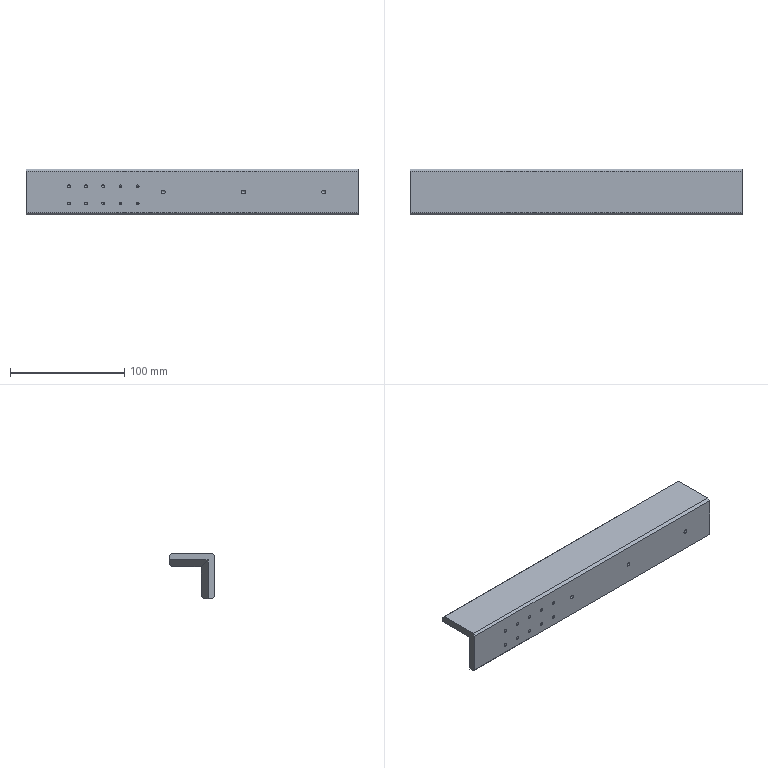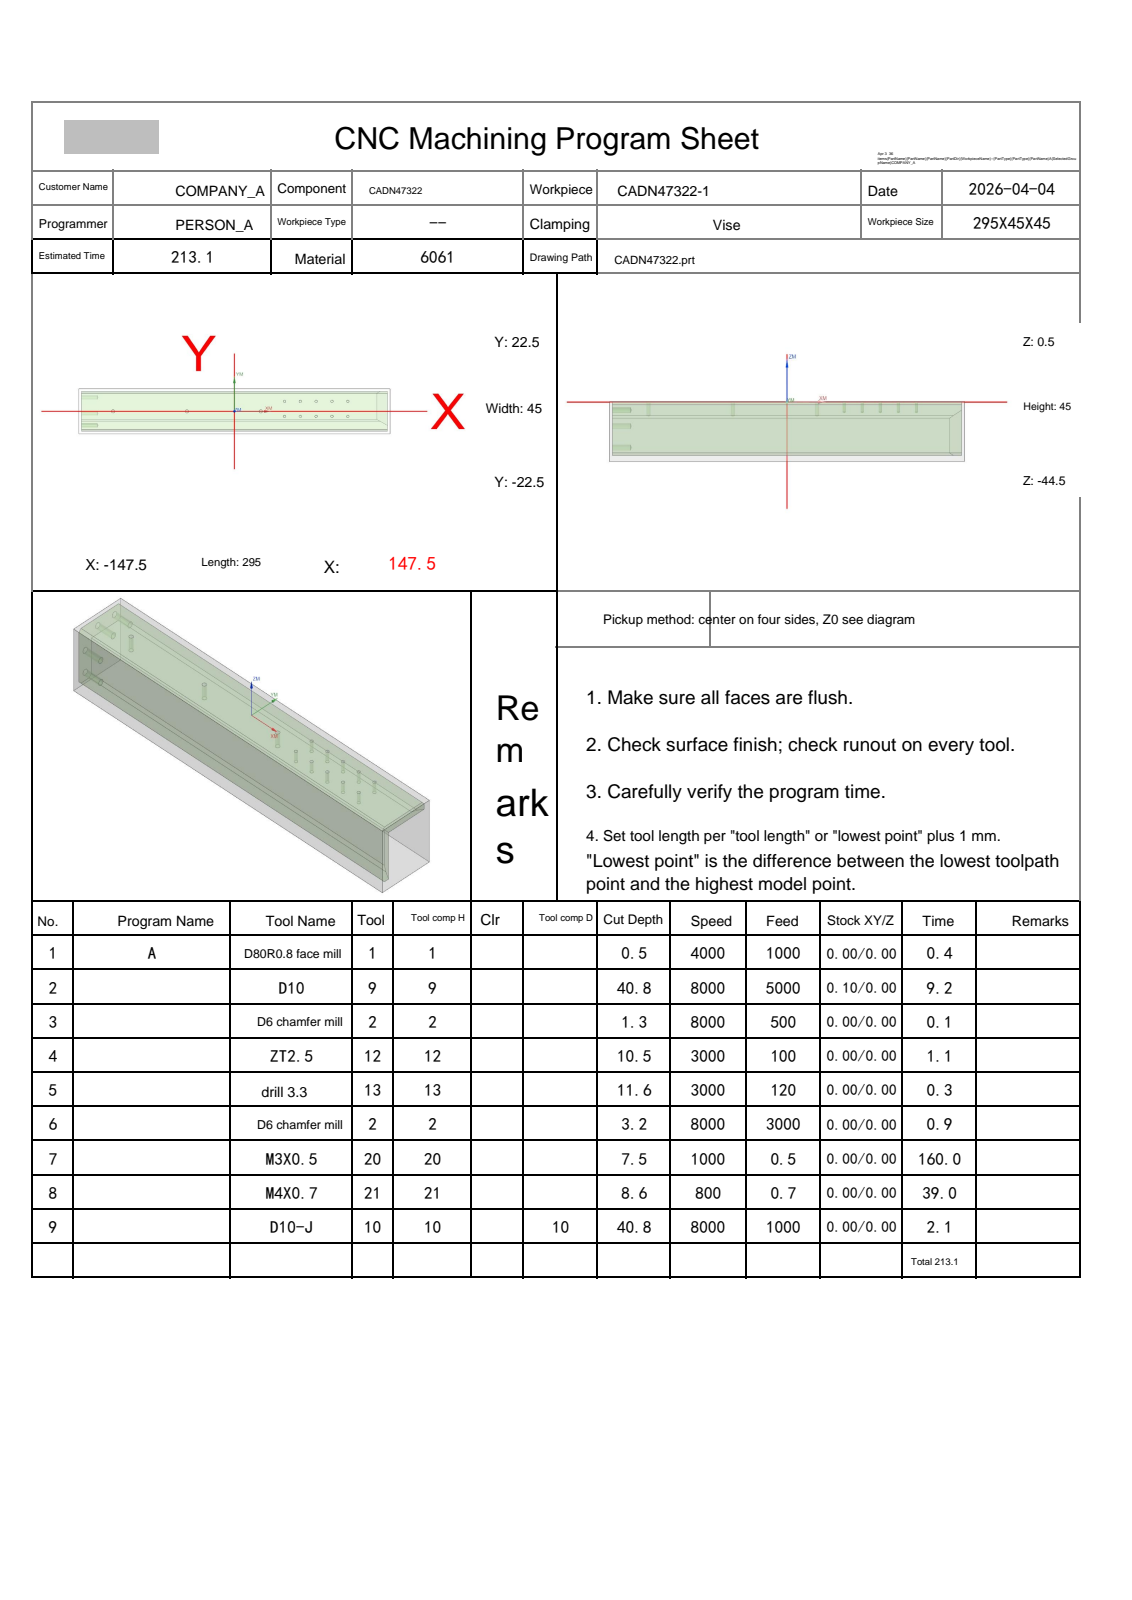NC program | NX | posted by the shop | part box 290 x 40 x 40 mm
Whole program:
%
O0001
(Machine time: 389.68 MIN)
(===Total Tool:8===)
(T1=D80R0.8 face mill D=80.  R=0.8  D-  H01 Z=0.    )
(T9=D10     D=10.  R=0.   D-  H09 Z=-40.3 )
(T2=D6 chamfer mill   D=6.   R=0.   D-  H02 Z=-2.7  )
(T12=ZT2.5  D=2.5  DR_a=118 D-  H12 Z=-10.  )
(T13=drill 3.3  D=3.3  DR_a=118 D-  H13 Z=-11.09)
(T20=M3X0.5 D=2.5  DR_a=180 D-  H20 Z=-7.   )
(T21=M4X0.7 D=3.3  DR_a=180 D-  H21 Z=-8.1  )
(T10=D10-J  D=10.  R=0.   D10 H10 Z=-40.3 )
G80 G90 G17 G49 G40
G91 G28 Z0
M01
N1 T01 M06
(D80R0.8 face mill  D=80. R=0.8 H=01 ce=0.00 di=0.00)
G00 G90 G54 X-190. Y0.0 M03 S4000
G43 H01 Z20.
M08
Z2.
G01 Z0.0 F1000.
X-185.
X185.
X190.
Z2.
G00 Z20.
G91 G28 Z0.0
M05
M09
G91 G28 Z0.0
M01
N2 T09 M06
(D10  D=10. R=0. H=09 ce=0.10 di=0.00)
G00 G90 G54 X0.0 Y-25.1 M03 S8000
G43 H09 Z20.
M08
Z.5
G01 X-145. Z.332 F5000.
G02 X-150.1 Y-20. Z.323 I0.0 J5.1
G01 Y20. Z.277
G02 X-145. Y25.1 Z.268 I5.1 J0.0
G01 X145. Z-.068
G02 X150.1 Y20. Z-.077 I0.0 J-5.1
G01 Y-20. Z-.123
G02 X145. Y-25.1 Z-.132 I-5.1 J0.0
G01 X-145. Z-.468
G02 X-150.1 Y-20. Z-.477 I0.0 J5.1
G01 Y20. Z-.523
G02 X-145. Y25.1 Z-.532 I5.1 J0.0
G01 X145. Z-.868
G02 X150.1 Y20. Z-.877 I0.0 J-5.1
G01 Y-20. Z-.923
G02 X145. Y-25.1 Z-.932 I-5.1 J0.0
G01 X-145. Z-1.268
G02 X-150.1 Y-20. Z-1.277 I0.0 J5.1
G01 Y20. Z-1.323
G02 X-145. Y25.1 Z-1.332 I5.1 J0.0
G01 X145. Z-1.668
G02 X150.1 Y20. Z-1.677 I0.0 J-5.1
G01 Y-20. Z-1.723
G02 X145. Y-25.1 Z-1.732 I-5.1 J0.0
G01 X-145. Z-2.068
G02 X-150.1 Y-20. Z-2.077 I0.0 J5.1
G01 Y20. Z-2.123
G02 X-145. Y25.1 Z-2.132 I5.1 J0.0
G01 X145. Z-2.468
G02 X150.1 Y20. Z-2.477 I0.0 J-5.1
G01 Y-20. Z-2.523
G02 X145. Y-25.1 Z-2.532 I-5.1 J0.0
G01 X-145. Z-2.868
G02 X-150.1 Y-20. Z-2.877 I0.0 J5.1
G01 Y20. Z-2.923
G02 X-145. Y25.1 Z-2.932 I5.1 J0.0
G01 X145. Z-3.268
G02 X150.1 Y20. Z-3.277 I0.0 J-5.1
G01 Y-20. Z-3.323
G02 X145. Y-25.1 Z-3.332 I-5.1 J0.0
G01 X-145. Z-3.668
G02 X-150.1 Y-20. Z-3.677 I0.0 J5.1
G01 Y20. Z-3.723
G02 X-145. Y25.1 Z-3.732 I5.1 J0.0
G01 X145. Z-4.068
G02 X150.1 Y20. Z-4.077 I0.0 J-5.1
G01 Y-20. Z-4.123
G02 X145. Y-25.1 Z-4.132 I-5.1 J0.0
G01 X-145. Z-4.468
G02 X-150.1 Y-20. Z-4.477 I0.0 J5.1
G01 Y20. Z-4.523
G02 X-145. Y25.1 Z-4.532 I5.1 J0.0
G01 X145. Z-4.868
G02 X150.1 Y20. Z-4.877 I0.0 J-5.1
G01 Y-20. Z-4.923
G02 X145. Y-25.1 Z-4.932 I-5.1 J0.0
G01 X-145. Z-5.268
G02 X-150.1 Y-20. Z-5.277 I0.0 J5.1
G01 Y20. Z-5.323
G02 X-145. Y25.1 Z-5.332 I5.1 J0.0
G01 X145. Z-5.668
G02 X150.1 Y20. Z-5.677 I0.0 J-5.1
G01 Y-20. Z-5.723
G02 X145. Y-25.1 Z-5.732 I-5.1 J0.0
G01 X-145. Z-6.068
G02 X-150.1 Y-20. Z-6.077 I0.0 J5.1
G01 Y20. Z-6.123
G02 X-145. Y25.1 Z-6.132 I5.1 J0.0
G01 X145. Z-6.468
G02 X150.1 Y20. Z-6.477 I0.0 J-5.1
G01 Y-20. Z-6.523
G02 X145. Y-25.1 Z-6.532 I-5.1 J0.0
G01 X-145. Z-6.868
G02 X-150.1 Y-20. Z-6.877 I0.0 J5.1
G01 Y20. Z-6.923
G02 X-145. Y25.1 Z-6.932 I5.1 J0.0
G01 X145. Z-7.268
G02 X150.1 Y20. Z-7.277 I0.0 J-5.1
G01 Y-20. Z-7.323
G02 X145. Y-25.1 Z-7.332 I-5.1 J0.0
G01 X-145. Z-7.668
G02 X-150.1 Y-20. Z-7.677 I0.0 J5.1
G01 Y20. Z-7.723
G02 X-145. Y25.1 Z-7.732 I5.1 J0.0
G01 X145. Z-8.068
G02 X150.1 Y20. Z-8.077 I0.0 J-5.1
G01 Y-20. Z-8.123
G02 X145. Y-25.1 Z-8.132 I-5.1 J0.0
G01 X-145. Z-8.468
G02 X-150.1 Y-20. Z-8.477 I0.0 J5.1
G01 Y20. Z-8.523
G02 X-145. Y25.1 Z-8.532 I5.1 J0.0
G01 X145. Z-8.868
G02 X150.1 Y20. Z-8.877 I0.0 J-5.1
G01 Y-20. Z-8.923
G02 X145. Y-25.1 Z-8.932 I-5.1 J0.0
G01 X-145. Z-9.268
G02 X-150.1 Y-20. Z-9.277 I0.0 J5.1
G01 Y20. Z-9.323
G02 X-145. Y25.1 Z-9.332 I5.1 J0.0
G01 X145. Z-9.668
G02 X150.1 Y20. Z-9.677 I0.0 J-5.1
G01 Y-20. Z-9.723
G02 X145. Y-25.1 Z-9.732 I-5.1 J0.0
G01 X-145. Z-10.068
G02 X-150.1 Y-20. Z-10.077 I0.0 J5.1
G01 Y20. Z-10.123
G02 X-145. Y25.1 Z-10.132 I5.1 J0.0
G01 X145. Z-10.468
G02 X150.1 Y20. Z-10.477 I0.0 J-5.1
G01 Y-20. Z-10.523
G02 X145. Y-25.1 Z-10.532 I-5.1 J0.0
G01 X-145. Z-10.868
G02 X-150.1 Y-20. Z-10.877 I0.0 J5.1
G01 Y20. Z-10.923
G02 X-145. Y25.1 Z-10.932 I5.1 J0.0
G01 X145. Z-11.268
G02 X150.1 Y20. Z-11.277 I0.0 J-5.1
G01 Y-20. Z-11.323
G02 X145. Y-25.1 Z-11.332 I-5.1 J0.0
G01 X-145. Z-11.668
G02 X-150.1 Y-20. Z-11.677 I0.0 J5.1
G01 Y20. Z-11.723
G02 X-145. Y25.1 Z-11.732 I5.1 J0.0
G01 X145. Z-12.068
G02 X150.1 Y20. Z-12.077 I0.0 J-5.1
G01 Y-20. Z-12.123
G02 X145. Y-25.1 Z-12.132 I-5.1 J0.0
G01 X-145. Z-12.468
G02 X-150.1 Y-20. Z-12.477 I0.0 J5.1
G01 Y20. Z-12.523
G02 X-145. Y25.1 Z-12.532 I5.1 J0.0
G01 X145. Z-12.868
G02 X150.1 Y20. Z-12.877 I0.0 J-5.1
G01 Y-20. Z-12.923
G02 X145. Y-25.1 Z-12.932 I-5.1 J0.0
G01 X-145. Z-13.268
G02 X-150.1 Y-20. Z-13.277 I0.0 J5.1
G01 Y20. Z-13.323
G02 X-145. Y25.1 Z-13.332 I5.1 J0.0
G01 X145. Z-13.668
G02 X150.1 Y20. Z-13.677 I0.0 J-5.1
G01 Y-20. Z-13.723
G02 X145. Y-25.1 Z-13.732 I-5.1 J0.0
G01 X-145. Z-14.068
G02 X-150.1 Y-20. Z-14.077 I0.0 J5.1
G01 Y20. Z-14.123
G02 X-145. Y25.1 Z-14.132 I5.1 J0.0
G01 X145. Z-14.468
G02 X150.1 Y20. Z-14.477 I0.0 J-5.1
G01 Y-20. Z-14.523
G02 X145. Y-25.1 Z-14.532 I-5.1 J0.0
G01 X-145. Z-14.868
G02 X-150.1 Y-20. Z-14.877 I0.0 J5.1
G01 Y20. Z-14.923
G02 X-145. Y25.1 Z-14.932 I5.1 J0.0
G01 X145. Z-15.268
G02 X150.1 Y20. Z-15.277 I0.0 J-5.1
G01 Y-20. Z-15.323
G02 X145. Y-25.1 Z-15.332 I-5.1 J0.0
G01 X-145. Z-15.668
G02 X-150.1 Y-20. Z-15.677 I0.0 J5.1
G01 Y20. Z-15.723
G02 X-145. Y25.1 Z-15.732 I5.1 J0.0
G01 X145. Z-16.068
G02 X150.1 Y20. Z-16.077 I0.0 J-5.1
G01 Y-20. Z-16.123
G02 X145. Y-25.1 Z-16.132 I-5.1 J0.0
G01 X-145. Z-16.468
G02 X-150.1 Y-20. Z-16.477 I0.0 J5.1
G01 Y20. Z-16.523
G02 X-145. Y25.1 Z-16.532 I5.1 J0.0
G01 X145. Z-16.868
G02 X150.1 Y20. Z-16.877 I0.0 J-5.1
G01 Y-20. Z-16.923
G02 X145. Y-25.1 Z-16.932 I-5.1 J0.0
G01 X-145. Z-17.268
G02 X-150.1 Y-20. Z-17.277 I0.0 J5.1
G01 Y20. Z-17.323
G02 X-145. Y25.1 Z-17.332 I5.1 J0.0
G01 X145. Z-17.668
G02 X150.1 Y20. Z-17.677 I0.0 J-5.1
G01 Y-20. Z-17.723
G02 X145. Y-25.1 Z-17.732 I-5.1 J0.0
G01 X-145. Z-18.068
G02 X-150.1 Y-20. Z-18.077 I0.0 J5.1
G01 Y20. Z-18.123
G02 X-145. Y25.1 Z-18.132 I5.1 J0.0
G01 X145. Z-18.468
G02 X150.1 Y20. Z-18.477 I0.0 J-5.1
G01 Y-20. Z-18.523
G02 X145. Y-25.1 Z-18.532 I-5.1 J0.0
G01 X-145. Z-18.868
G02 X-150.1 Y-20. Z-18.877 I0.0 J5.1
G01 Y20. Z-18.923
G02 X-145. Y25.1 Z-18.932 I5.1 J0.0
G01 X145. Z-19.268
G02 X150.1 Y20. Z-19.277 I0.0 J-5.1
G01 Y-20. Z-19.323
G02 X145. Y-25.1 Z-19.332 I-5.1 J0.0
G01 X-145. Z-19.668
G02 X-150.1 Y-20. Z-19.677 I0.0 J5.1
G01 Y20. Z-19.723
G02 X-145. Y25.1 Z-19.732 I5.1 J0.0
G01 X145. Z-20.068
G02 X150.1 Y20. Z-20.077 I0.0 J-5.1
G01 Y-20. Z-20.123
G02 X145. Y-25.1 Z-20.132 I-5.1 J0.0
G01 X-145. Z-20.468
G02 X-150.1 Y-20. Z-20.477 I0.0 J5.1
G01 Y20. Z-20.523
G02 X-145. Y25.1 Z-20.532 I5.1 J0.0
G01 X145. Z-20.868
G02 X150.1 Y20. Z-20.877 I0.0 J-5.1
G01 Y-20. Z-20.923
G02 X145. Y-25.1 Z-20.932 I-5.1 J0.0
G01 X-145. Z-21.268
G02 X-150.1 Y-20. Z-21.277 I0.0 J5.1
G01 Y20. Z-21.323
G02 X-145. Y25.1 Z-21.332 I5.1 J0.0
G01 X145. Z-21.668
G02 X150.1 Y20. Z-21.677 I0.0 J-5.1
G01 Y-20. Z-21.723
G02 X145. Y-25.1 Z-21.732 I-5.1 J0.0
G01 X-145. Z-22.068
G02 X-150.1 Y-20. Z-22.077 I0.0 J5.1
G01 Y20. Z-22.123
G02 X-145. Y25.1 Z-22.132 I5.1 J0.0
G01 X145. Z-22.468
G02 X150.1 Y20. Z-22.477 I0.0 J-5.1
G01 Y-20. Z-22.523
G02 X145. Y-25.1 Z-22.532 I-5.1 J0.0
G01 X-145. Z-22.868
G02 X-150.1 Y-20. Z-22.877 I0.0 J5.1
G01 Y20. Z-22.923
G02 X-145. Y25.1 Z-22.932 I5.1 J0.0
G01 X145. Z-23.268
G02 X150.1 Y20. Z-23.277 I0.0 J-5.1
G01 Y-20. Z-23.323
G02 X145. Y-25.1 Z-23.332 I-5.1 J0.0
G01 X-145. Z-23.668
G02 X-150.1 Y-20. Z-23.677 I0.0 J5.1
G01 Y20. Z-23.723
G02 X-145. Y25.1 Z-23.732 I5.1 J0.0
G01 X145. Z-24.068
G02 X150.1 Y20. Z-24.077 I0.0 J-5.1
G01 Y-20. Z-24.123
G02 X145. Y-25.1 Z-24.132 I-5.1 J0.0
G01 X-145. Z-24.468
G02 X-150.1 Y-20. Z-24.477 I0.0 J5.1
G01 Y20. Z-24.523
G02 X-145. Y25.1 Z-24.532 I5.1 J0.0
G01 X145. Z-24.868
G02 X150.1 Y20. Z-24.877 I0.0 J-5.1
G01 Y-20. Z-24.923
G02 X145. Y-25.1 Z-24.932 I-5.1 J0.0
G01 X-145. Z-25.268
G02 X-150.1 Y-20. Z-25.277 I0.0 J5.1
G01 Y20. Z-25.323
G02 X-145. Y25.1 Z-25.332 I5.1 J0.0
G01 X145. Z-25.668
G02 X150.1 Y20. Z-25.677 I0.0 J-5.1
G01 Y-20. Z-25.723
G02 X145. Y-25.1 Z-25.732 I-5.1 J0.0
G01 X-145. Z-26.068
G02 X-150.1 Y-20. Z-26.077 I0.0 J5.1
G01 Y20. Z-26.123
G02 X-145. Y25.1 Z-26.132 I5.1 J0.0
G01 X145. Z-26.468
G02 X150.1 Y20. Z-26.477 I0.0 J-5.1
G01 Y-20. Z-26.523
G02 X145. Y-25.1 Z-26.532 I-5.1 J0.0
G01 X-145. Z-26.868
G02 X-150.1 Y-20. Z-26.877 I0.0 J5.1
G01 Y20. Z-26.923
G02 X-145. Y25.1 Z-26.932 I5.1 J0.0
G01 X145. Z-27.268
G02 X150.1 Y20. Z-27.277 I0.0 J-5.1
G01 Y-20. Z-27.323
G02 X145. Y-25.1 Z-27.332 I-5.1 J0.0
G01 X-145. Z-27.668
G02 X-150.1 Y-20. Z-27.677 I0.0 J5.1
G01 Y20. Z-27.723
G02 X-145. Y25.1 Z-27.732 I5.1 J0.0
G01 X145. Z-28.068
G02 X150.1 Y20. Z-28.077 I0.0 J-5.1
G01 Y-20. Z-28.123
G02 X145. Y-25.1 Z-28.132 I-5.1 J0.0
G01 X-145. Z-28.468
G02 X-150.1 Y-20. Z-28.477 I0.0 J5.1
G01 Y20. Z-28.523
G02 X-145. Y25.1 Z-28.532 I5.1 J0.0
G01 X145. Z-28.868
G02 X150.1 Y20. Z-28.877 I0.0 J-5.1
G01 Y-20. Z-28.923
G02 X145. Y-25.1 Z-28.932 I-5.1 J0.0
G01 X-145. Z-29.268
G02 X-150.1 Y-20. Z-29.277 I0.0 J5.1
G01 Y20. Z-29.323
G02 X-145. Y25.1 Z-29.332 I5.1 J0.0
G01 X145. Z-29.668
G02 X150.1 Y20. Z-29.677 I0.0 J-5.1
G01 Y-20. Z-29.723
G02 X145. Y-25.1 Z-29.732 I-5.1 J0.0
G01 X-145. Z-30.068
G02 X-150.1 Y-20. Z-30.077 I0.0 J5.1
G01 Y20. Z-30.123
G02 X-145. Y25.1 Z-30.132 I5.1 J0.0
G01 X145. Z-30.468
G02 X150.1 Y20. Z-30.477 I0.0 J-5.1
G01 Y-20. Z-30.523
G02 X145. Y-25.1 Z-30.532 I-5.1 J0.0
G01 X-145. Z-30.868
G02 X-150.1 Y-20. Z-30.877 I0.0 J5.1
G01 Y20. Z-30.923
G02 X-145. Y25.1 Z-30.932 I5.1 J0.0
G01 X145. Z-31.268
G02 X150.1 Y20. Z-31.277 I0.0 J-5.1
G01 Y-20. Z-31.323
G02 X145. Y-25.1 Z-31.332 I-5.1 J0.0
G01 X-145. Z-31.668
G02 X-150.1 Y-20. Z-31.677 I0.0 J5.1
G01 Y20. Z-31.723
G02 X-145. Y25.1 Z-31.732 I5.1 J0.0
G01 X145. Z-32.068
G02 X150.1 Y20. Z-32.077 I0.0 J-5.1
G01 Y-20. Z-32.123
G02 X145. Y-25.1 Z-32.132 I-5.1 J0.0
G01 X-145. Z-32.468
G02 X-150.1 Y-20. Z-32.477 I0.0 J5.1
G01 Y20. Z-32.523
G02 X-145. Y25.1 Z-32.532 I5.1 J0.0
G01 X145. Z-32.868
G02 X150.1 Y20. Z-32.877 I0.0 J-5.1
G01 Y-20. Z-32.923
G02 X145. Y-25.1 Z-32.932 I-5.1 J0.0
G01 X-145. Z-33.268
G02 X-150.1 Y-20. Z-33.277 I0.0 J5.1
G01 Y20. Z-33.323
G02 X-145. Y25.1 Z-33.332 I5.1 J0.0
G01 X145. Z-33.668
G02 X150.1 Y20. Z-33.677 I0.0 J-5.1
G01 Y-20. Z-33.723
G02 X145. Y-25.1 Z-33.732 I-5.1 J0.0
G01 X-145. Z-34.068
G02 X-150.1 Y-20. Z-34.077 I0.0 J5.1
G01 Y20. Z-34.123
G02 X-145. Y25.1 Z-34.132 I5.1 J0.0
G01 X145. Z-34.468
G02 X150.1 Y20. Z-34.477 I0.0 J-5.1
G01 Y-20. Z-34.523
G02 X145. Y-25.1 Z-34.532 I-5.1 J0.0
G01 X-145. Z-34.868
G02 X-150.1 Y-20. Z-34.877 I0.0 J5.1
G01 Y20. Z-34.923
G02 X-145. Y25.1 Z-34.932 I5.1 J0.0
G01 X145. Z-35.268
G02 X150.1 Y20. Z-35.277 I0.0 J-5.1
G01 Y-20. Z-35.323
G02 X145. Y-25.1 Z-35.332 I-5.1 J0.0
G01 X-145. Z-35.668
G02 X-150.1 Y-20. Z-35.677 I0.0 J5.1
G01 Y20. Z-35.723
G02 X-145. Y25.1 Z-35.732 I5.1 J0.0
G01 X145. Z-36.068
G02 X150.1 Y20. Z-36.077 I0.0 J-5.1
G01 Y-20. Z-36.123
G02 X145. Y-25.1 Z-36.132 I-5.1 J0.0
G01 X-145. Z-36.468
G02 X-150.1 Y-20. Z-36.477 I0.0 J5.1
G01 Y20. Z-36.523
G02 X-145. Y25.1 Z-36.532 I5.1 J0.0
G01 X145. Z-36.868
G02 X150.1 Y20. Z-36.877 I0.0 J-5.1
G01 Y-20. Z-36.923
G02 X145. Y-25.1 Z-36.932 I-5.1 J0.0
G01 X-145. Z-37.268
G02 X-150.1 Y-20. Z-37.277 I0.0 J5.1
G01 Y20. Z-37.323
G02 X-145. Y25.1 Z-37.332 I5.1 J0.0
G01 X145. Z-37.668
G02 X150.1 Y20. Z-37.677 I0.0 J-5.1
G01 Y-20. Z-37.723
G02 X145. Y-25.1 Z-37.732 I-5.1 J0.0
G01 X-145. Z-38.068
G02 X-150.1 Y-20. Z-38.077 I0.0 J5.1
G01 Y20. Z-38.123
G02 X-145. Y25.1 Z-38.132 I5.1 J0.0
G01 X145. Z-38.468
G02 X150.1 Y20. Z-38.477 I0.0 J-5.1
G01 Y-20. Z-38.523
G02 X145. Y-25.1 Z-38.532 I-5.1 J0.0
G01 X-145. Z-38.868
G02 X-150.1 Y-20. Z-38.877 I0.0 J5.1
G01 Y20. Z-38.923
G02 X-145. Y25.1 Z-38.932 I5.1 J0.0
G01 X145. Z-39.268
G02 X150.1 Y20. Z-39.277 I0.0 J-5.1
G01 Y-20. Z-39.323
G02 X145. Y-25.1 Z-39.332 I-5.1 J0.0
G01 X-145. Z-39.668
G02 X-150.1 Y-20. Z-39.677 I0.0 J5.1
G01 Y20. Z-39.723
G02 X-145. Y25.1 Z-39.732 I5.1 J0.0
G01 X145. Z-40.068
G02 X150.1 Y20. Z-40.077 I0.0 J-5.1
G01 Y-20. Z-40.123
G02 X145. Y-25.1 Z-40.132 I-5.1 J0.0
G01 X0.0 Z-40.3
X-145.
G02 X-150.1 Y-20. I0.0 J5.1
G01 Y20.
G02 X-145. Y25.1 I5.1 J0.0
G01 X145.
G02 X150.1 Y20. I0.0 J-5.1
G01 Y-20.
G02 X145. Y-25.1 I-5.1 J0.0
G01 X0.0
X-.5
Z-39.3
G00 Z20.
G00 G90 X-154.936 Y22.983 M03 S7000
Z10.878
Z.359
G01 Z-.141 F4500.
X-146.072 Y23.239
X-145.985 Y23.241
X145.985
X146.072 Y23.239
Y23.312 Z-.212
Y23.38 Z-.283
X145.985 Y23.383
X-145.985
X-146.072 Y23.38
Y23.454 Z-.354
Y23.522 Z-.424
X-145.985 Y23.524
X145.985
X146.072 Y23.522
Y23.595 Z-.495
X146.073 Y23.663 Z-.566
X145.985 Y23.666
X-145.985
X-146.073 Y23.663
Y23.736 Z-.636
Y23.805 Z-.707
X-145.985 Y23.807
X145.985
X146.073 Y23.805
Y23.878 Z-.778
Y23.946 Z-.849
X145.985 Y23.949
X-145.985
X-146.073 Y23.946
Y24.019 Z-.919
Y24.087 Z-.99
X-145.985 Y24.09
X145.985
X146.073 Y24.087
Y24.161 Z-1.061
Y24.229 Z-1.131
X145.985 Y24.231
X-145.985
X-146.073 Y24.229
Y24.302 Z-1.202
Y24.37 Z-1.273
X-145.985 Y24.373
X145.985
X146.073 Y24.37
Y24.444 Z-1.344
Y24.512 Z-1.414
X145.985 Y24.514
X-145.985
X-146.073 Y24.512
X-146.072 Y24.585 Z-1.485
Y24.653 Z-1.556
X-145.985 Y24.656
X145.985
X146.072 Y24.653
Y24.711 Z-1.611
Y24.764 Z-1.667
X145.985 Y24.767
X-145.985
X-146.072 Y24.764
Y24.822 Z-1.722
Y24.875 Z-1.778
X-145.985 Y24.878
X145.985
X146.072 Y24.875
Y24.933 Z-1.833
Y24.986 Z-1.889
X145.985 Y24.989
X-145.985
X-146.072 Y24.986
Y25.044 Z-1.944
Y25.097 Z-2.
X146.072
G00 Z10.878
X154.934 Y-22.983
Z.359
G01 Z-.141
X146.072 Y-23.239
X145.985 Y-23.241
X-145.985
X-146.072 Y-23.239
Y-23.312 Z-.212
Y-23.38 Z-.283
X-145.985 Y-23.383
X145.985
X146.072 Y-23.38
Y-23.454 Z-.354
Y-23.522 Z-.424
X145.985 Y-23.524
X-145.985
X-146.072 Y-23.522
Y-23.595 Z-.495
X-146.073 Y-23.663 Z-.566
X-145.985 Y-23.666
X145.985
X146.073 Y-23.663
Y-23.736 Z-.636
Y-23.805 Z-.707
X145.985 Y-23.807
X-145.985
X-146.073 Y-23.805
Y-23.878 Z-.778
Y-23.946 Z-.849
X-145.985 Y-23.949
X145.985
X146.073 Y-23.946
Y-24.019 Z-.919
Y-24.087 Z-.99
X145.985 Y-24.09
X-145.985
X-146.073 Y-24.087
Y-24.161 Z-1.061
Y-24.229 Z-1.131
X-145.985 Y-24.231
X145.985
X146.073 Y-24.229
Y-24.302 Z-1.202
Y-24.37 Z-1.273
X145.985 Y-24.373
X-145.985
X-146.073 Y-24.37
Y-24.444 Z-1.344
Y-24.512 Z-1.414
X-145.985 Y-24.514
X145.985
X146.073 Y-24.512
X146.072 Y-24.585 Z-1.485
Y-24.653 Z-1.556
X145.985 Y-24.656
X-145.985
X-146.072 Y-24.653
Y-24.711 Z-1.611
Y-24.764 Z-1.667
X-145.985 Y-24.767
X145.985
X146.072 Y-24.764
Y-24.822 Z-1.722
Y-24.875 Z-1.778
X145.985 Y-24.878
X-145.985
X-146.072 Y-24.875
Y-24.933 Z-1.833
Y-24.986 Z-1.889
X-145.985 Y-24.989
X145.985
X146.072 Y-24.986
Y-25.044 Z-1.944
Y-25.097 Z-2.
X-146.072
G00 Z10.878
G91 G28 Z0.0
M05
M09
G91 G28 Z0.0
M01
N3 T02 M06
(D6 chamfer mill  D=6. R=0. H=02 ce=0.00 di=0.00)
G00 G90 G54 X77.5 Y-5. M03 S8000
G43 H02 Z20.
M08
G98 G81 X77.5 Y-5. Z-.8 R1. F500.
X92.5
X107.5
Y10.
X92.5
X77.5
X62.5
Y-5.
X47.5
Y10.
X25. Y0.0
X-45.
X-115.
G80
G00 Z20.
G91 G28 Z0.0
M05
M09
G91 G28 Z0.0
M01
N4 T12 M06
(ZT2.5 D=2.5 DR_a=118 H=12)
G00 G90 G54 X62.5 Y10. M03 S3000
G43 H12 Z20.
M08
G98 G83 X62.5 Y10. Z-10. R1. F100. Q2.
X47.5
Y-5.
X62.5
X77.5
Y10.
X92.5
Y-5.
X107.5
Y10.
G80
G00 Z20.
G91 G28 Z0.0
M05
M09
G91 G28 Z0.0
M01
N5 T13 M06
(drill 3.3 D=3.3 DR_a=118 H=13)
G00 G90 G54 X-115. Y0.0 M03 S3000
G43 H13 Z20.
M08
G98 G83 X-115. Y0.0 Z-11.091 R1. F120. Q2.
X-45.
X25.
G80
G00 Z20.
G91 G28 Z0.0
M05
M09
G91 G28 Z0.0
M01
N6 T02 M06
(D6 chamfer mill  D=6. R=0. H=02 ce=0.00 di=0.00)
G00 G90 G54 X-146.207 Y-18.461 M03 S8000
G43 H02 Z20.
M08
Z2.935
G01 Z-1.5 F3000.
X-146.267 Y-18.289
X-146.3 Y-18.
Y18.
X-146.267 Y18.289
X-146.207 Y18.461
Z2.935
G00 Z20.
X146.207
Z2.935
G01 Z-1.5
X146.267 Y18.289
X146.3 Y18.
Y-18.
X146.267 Y-18.289
X146.207 Y-18.461
Z2.935
G00 Z20.
G00 G90 X-148.9 Y21.516 M03 S6500
Z20.
Z-1.2
G01 Z-2.7 F1000.
G03 X-147.763 Y20.7 I1.137 J.384
G01 X147.763
G03 X148.9 Y21.516 I0.0 J1.2
G01 Z-1.2
G00 Z20.
Y-21.516
Z-1.2
G01 Z-2.7
G03 X147.763 Y-20.7 I-1.137 J-.384
G01 X-147.763
G03 X-148.9 Y-21.516 I0.0 J-1.2
G01 Z-1.2
G00 Z20.
G00 G90 X62.5 Y10. M03 S8000
Z20.
G98 G81 X62.5 Y10. Z-1.75 R3. F500.
X47.5
Y-5.
X62.5
X77.5
Y10.
X92.5
Y-5.
X107.5
Y10.
G80
G00 Z20.
G00 G90 X-115. Y0.0 M03 S8000
Z20.
G98 G81 X-115. Y0.0 Z-2.2 R3. F500.
X-45.
X25.
G80
G00 Z20.
G91 G28 Z0.0
M05
M09
G91 G28 Z0.0
M01
N7 T20 M06
(M3X0.5 D=2.5 DR_a=180 H=20)
G00 G90 G54 X62.5 Y10. M03 S1000
G43 H20 Z20.
M08
G95
G98 G84 X62.5 Y10. Z-7. R1. F.5 Q2.
X47.5
Y-5.
X62.5
X77.5
Y10.
X92.5
Y-5.
X107.5
Y10.
G80
G94
G00 Z20.
G91 G28 Z0.0
M05
M09
G91 G28 Z0.0
M01
N8 T21 M06
(M4X0.7 D=3.3 DR_a=180 H=21)
G00 G90 G54 X-115. Y0.0 M03 S800
G43 H21 Z20.
M08
G95
G98 G84 X-115. Y0.0 Z-8.1 R1. F.7 Q3.
X-45.
X25.
G80
G94
G00 Z20.
G91 G28 Z0.0
M05
M09
G91 G28 Z0.0
M01
N9 T10 M06
(D10-J  D=10. R=0. H=10 ce=0.00 di=0.00)
G00 G90 G54 X-146.013 Y26.116 M03 S8000
G43 H10 Z20.
M08
Z-12.933
G01 Z-13.433 F1000.
G41 D10
X-145.997 Y25.917
G03 X-145. Y25. I.997 J.083
G01 X145.
G02 X150. Y20. I0.0 J-5.
G01 Y-20.
G02 X145. Y-25. I-5. J0.0
G01 X-145.
G02 X-150. Y-20. I0.0 J5.
G01 Y20.
G02 X-145. Y25. I5. J0.0
G01 X-144.5
G03 X-143.5 Y26. I0.0 J1.
G01 G40 Y26.2
Z-12.933
G00 Z20.
X-146.013 Y26.116
Z-26.367
G01 Z-26.867
G41 D10
X-145.997 Y25.917
G03 X-145. Y25. I.997 J.083
G01 X145.
G02 X150. Y20. I0.0 J-5.
G01 Y-20.
G02 X145. Y-25. I-5. J0.0
G01 X-145.
G02 X-150. Y-20. I0.0 J5.
G01 Y20.
G02 X-145. Y25. I5. J0.0
G01 X-144.5
G03 X-143.5 Y26. I0.0 J1.
G01 G40 Y26.2
Z-26.367
G00 Z20.
X-146.013 Y26.116
Z-39.8
G01 Z-40.3
G41 D10
X-145.997 Y25.917
G03 X-145. Y25. I.997 J.083
G01 X145.
G02 X150. Y20. I0.0 J-5.
G01 Y-20.
G02 X145. Y-25. I-5. J0.0
G01 X-145.
G02 X-150. Y-20. I0.0 J5.
G01 Y20.
G02 X-145. Y25. I5. J0.0
G01 X-144.5
G03 X-143.5 Y26. I0.0 J1.
G01 G40 Y26.2
Z-39.8
G00 Z20.
M05
M09
G91 G28 Z0.0
G91 G28 Y0.0
M30
%